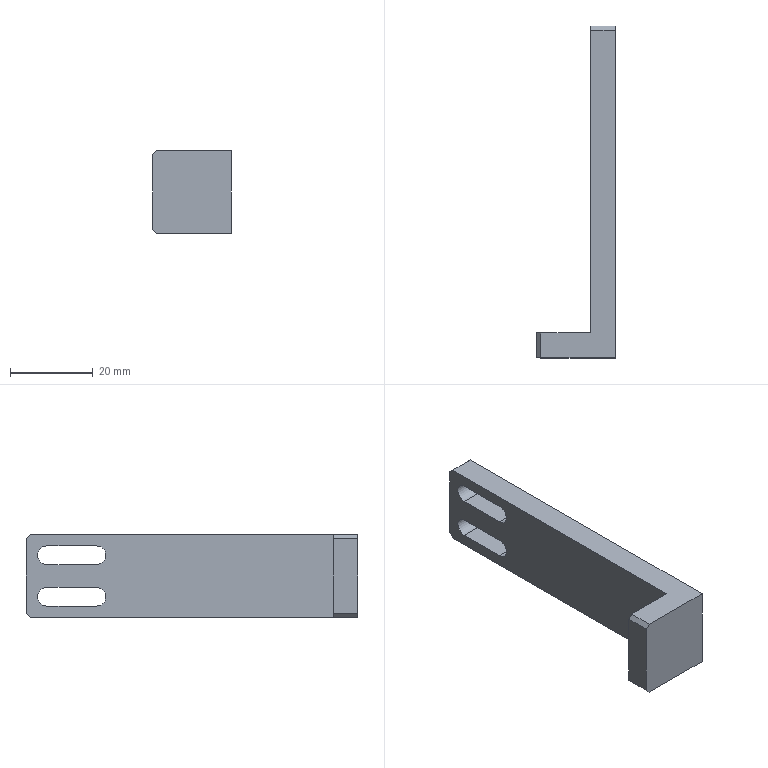Part | STEP file | 0-19-08 Cover plate block | 1 solid | 20 faces | box 19 x 80 x 20 mm | volume 10309 mm3 | plane 16 | cylinder 4 | commonest cylinder face diameters 4.5 x4